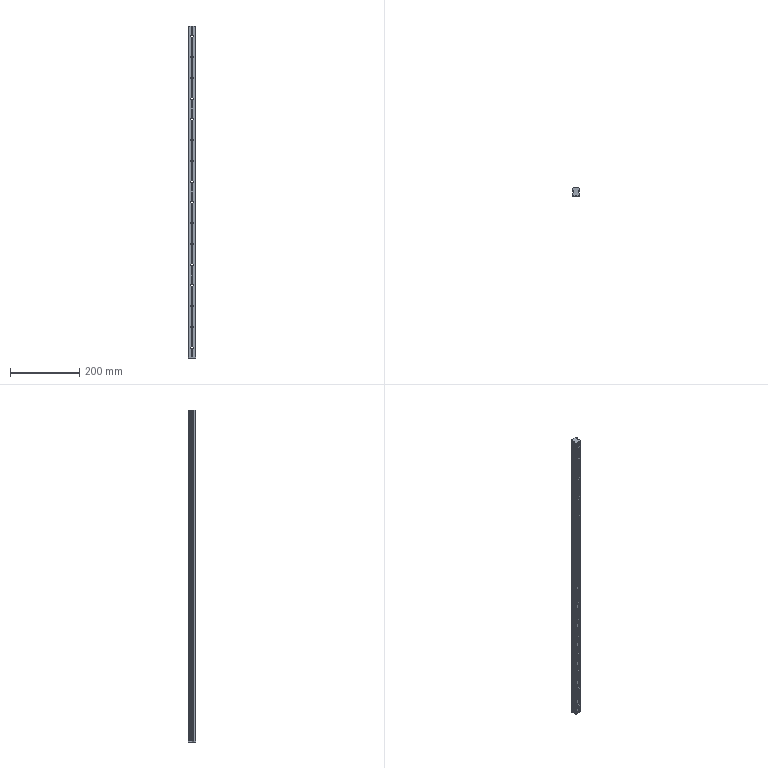Part | SolidWorks | features BaseBody 1 | 1 solid | 285 faces | box 23 x 22 x 960 mm | volume 392872 mm3 | plane 156 | cylinder 72 | spline 57 | commonest cylinder face diameters 7 x32 11 x32 2 x4 4.6 x4